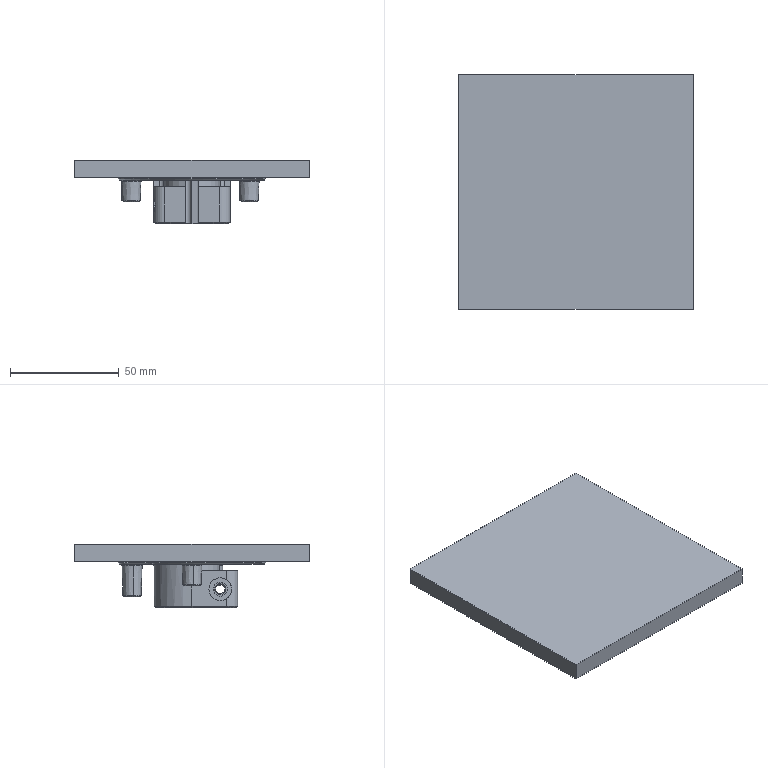NC program | NX | posted with a generic post | part box 108 x 108 x 29 mm
Lines 1 to 1353 of 23883:
N10 G17 G21 G94 G90
(FLOOR_WALL_COPY_COPY , TOOL : D63)
N12 T03 M6
N14 G54
N16 G17 G0 G90 X-68.5 Y33.999 S6500 M3
N18 G43 Z30. H3
N20 Z7.03
N22 G94 G1 Z4.03 F1250.
N24 X-65.5
N26 X65.5
N28 Y-8.8
N30 X-65.5
N32 X-68.5
N34 Z7.03
N36 G0 Z30.
N38 Y33.999
N40 Z6.06
N42 G1 Z3.06
N44 X-65.5
N46 X65.5
N48 Y-8.8
N50 X-65.5
N52 X-68.5
N54 Z6.06
N56 G0 Z30.
N58 Y33.999
N60 Z5.09
N62 G1 Z2.09
N64 X-65.5
N66 X65.5
N68 Y-8.8
N70 X-65.5
N72 X-68.5
N74 Z5.09
N76 G0 Z30.
N78 Y33.999
N80 Z4.12
N82 G1 Z1.12
N84 X-65.5
N86 X65.5
N88 Y-8.8
N90 X-65.5
N92 X-68.5
N94 Z4.12
N96 G0 Z30.
N98 Y33.999
N100 Z3.15
N102 G1 Z0.15
N104 X-65.5
N106 X65.5
N108 Y-8.8
N110 X-65.5
N112 X-68.5
N114 Z3.15
N116 G0 Z30.
(FLOOR_WALL_COPY_COPY_1 , TOOL : D63)
N118 X-68.499 Y33.998
N120 Z3.
N122 G1 Z0.
N124 X-65.499
N126 X65.499
N128 Y-8.799
N130 X-65.499
N132 X-68.499
N134 Z3.
N136 G0 Z30.
N138 M5
(CAVITY_MILL , TOOL : D10)
N140 T04 M6
N142 G54
N144 G17 G0 G90 X-40.997 Y12.31 S9500 M3
N146 G43 Z30. H4
N148 Z0.52
N150 G94 G1 Z-0.98 F1000.
N152 X-34.997 Y15.774
N154 G3 X-34.497 Y16.64 R1.
N156 G1 X-28.497
N158 Y2.421 F2500.
N160 X-28.709 Y-2.575
N162 G3 X-27.6 Y-2.498 R5.
N164 G1 Y-16.
N166 G3 X-26.755 Y-20.98 R15.1
N168 G2 X-29.497 Y-16.909 R34.
N170 G1 Y-2.478
N172 G3 X-28.709 Y-2.575 R5.
N174 G1 X-28.497 Y2.421
N176 G2 X-2.421 Y28.497 R28.6
N178 G1 X-16.64
N180 G3 X-28.497 Y16.64 R33.
N182 G1 X-34.497
N184 Y-18.192
N186 G3 X-18.192 Y-34.497 R39.
N188 G1 X18.192
N190 G3 X34.497 Y-18.192 R39.
N192 G1 Y2.421
N194 X28.497
N196 Y16.639
N198 G3 X25.153 Y16.744 R2.
N200 G1 X24.153 Y15.316
N202 G2 X28.497 Y2.421 R28.6
N204 G1 X28.709 Y-2.575
N206 G3 X29.497 Y-2.478 R5.
N208 G1 Y-16.909
N210 G2 X26.755 Y-20.98 R34.
N212 G3 X27.6 Y-16. R15.1
N214 G1 Y-2.498
N216 G3 X28.709 Y-2.575 R5.
N218 G1 X28.497 Y2.421
N220 X34.497
N222 Y18.192
N224 G3 X33.705 Y19.621 R39.
N226 X20.238 Y20.185 R8.
N228 G1 X16.737 Y15.186
N230 G2 X22.6 Y0. R22.6
N232 G1 Y-16.
N234 G2 X12.5 Y-26.1 R10.1
N236 G1 X3.
N238 G2 X0. Y-25.124 R5.1
N240 G1 X-0.067 Y-25.172
N242 G2 X-3. Y-26.1 R5.1
N244 G1 X-12.5
N246 G2 X-22.6 Y-16. R10.1
N248 G1 Y0.
N250 G2 X1.913 Y22.519 R22.6
N252 G1 X2.421 Y28.497
N254 G2 X6.132 Y27.935 R28.6
N256 G1 X6.526 Y28.497
N258 X2.421
N260 X1.913 Y22.519
N262 G2 X4.881 Y22.067 R22.6
N264 X8.546 Y20.922 R22.601
N266 G1 X12.046 Y25.921
N268 G3 X12.428 Y34.497 R8.
N270 G1 X-18.192
N272 G3 X-34.497 Y18.192 R39.
N274 G1 Y16.64
N276 G2 X-34.997 Y15.774 R1.
N278 G1 X-40.997 Y12.31
N280 Z0.52
N282 G0 Z-0.46
N284 G1 Z-1.96 F1000.
N286 X-34.997 Y15.774
N288 G3 X-34.497 Y16.64 R1.
N290 G1 X-28.497
N292 Y2.42 F2500.
N294 X-27.6 Y-2.499
N296 Y-16.
N298 G3 X-26.755 Y-20.98 R15.1
N300 G2 X-29.497 Y-16.909 R34.
N302 G1 Y-2.479
N304 G3 X-27.6 Y-2.499 R5.
N306 G1 X-28.497 Y2.42
N308 G2 X-2.42 Y28.497 R28.6
N310 G1 X-16.64
N312 G3 X-28.497 Y16.64 R33.
N314 G1 X-34.497
N316 Y-18.191
N318 G3 X-18.191 Y-34.497 R39.
N320 G1 X18.191
N322 G3 X34.497 Y-18.191 R39.
N324 G1 Y2.42
N326 X28.497
N328 Y16.639
N330 G3 X25.153 Y16.744 R2.
N332 G1 X24.153 Y15.316
N334 G2 X28.497 Y2.42 R28.6
N336 G1 X28.709 Y-2.576
N338 G3 X29.497 Y-2.479 R5.
N340 G1 Y-16.909
N342 G2 X26.755 Y-20.98 R34.
N344 G3 X27.6 Y-16. R15.1
N346 G1 Y-2.499
N348 G3 X28.709 Y-2.576 R5.
N350 G1 X28.497 Y2.42
N352 X34.497
N354 Y18.191
N356 G3 X33.705 Y19.621 R39.
N358 X20.238 Y20.185 R8.
N360 G1 X16.737 Y15.186
N362 G2 X22.6 Y0. R22.6
N364 G1 Y-16.
N366 G2 X12.5 Y-26.1 R10.1
N368 G1 X3.
N370 G2 X0. Y-25.124 R5.1
N372 G1 X-0.067 Y-25.172
N374 G2 X-3. Y-26.1 R5.1
N376 G1 X-12.5
N378 G2 X-22.6 Y-16. R10.1
N380 G1 Y0.
N382 G2 X1.912 Y22.519 R22.6
N384 G1 X2.42 Y28.497
N386 G2 X6.132 Y27.935 R28.6
N388 G1 X6.526 Y28.497
N390 X2.42
N392 X1.912 Y22.519
N394 G2 X5.91 Y21.813 R22.6
N396 X8.546 Y20.922 R22.601
N398 G1 X12.046 Y25.921
N400 G3 X12.428 Y34.497 R8.
N402 G1 X-18.191
N404 G3 X-34.497 Y18.191 R39.
N406 G1 Y16.64
N408 G2 X-34.997 Y15.774 R1.
N410 G1 X-40.997 Y12.31
N412 Z-0.46
N414 G0 X-40.998 Z-1.44
N416 G1 Z-2.94 F1000.
N418 X-34.998 Y15.774
N420 G3 X-34.498 Y16.64 R1.
N422 G1 X-28.498
N424 Y2.418 F2500.
N426 X-28.709 Y-2.577
N428 G3 X-27.6 Y-2.5 R5.
N430 G1 Y-16.
N432 G3 X-26.755 Y-20.98 R15.1
N434 G2 X-29.498 Y-16.908 R34.
N436 G1 Y-2.481
N438 G3 X-28.709 Y-2.577 R5.
N440 G1 X-28.498 Y2.418
N442 G2 X-2.418 Y28.498 R28.6
N444 G1 X-16.64
N446 G3 X-28.498 Y16.64 R33.
N448 G1 X-33.679 Y19.665
N450 G3 X-34.498 Y18.191 R39.
N452 G1 Y-18.191
N454 G3 X-18.191 Y-34.498 R39.
N456 G1 X18.191
N458 G3 X34.498 Y-18.191 R39.
N460 G1 Y2.418
N462 X28.498
N464 Y16.639
N466 G3 X25.153 Y16.744 R2.
N468 G1 X24.153 Y15.316
N470 G2 X28.498 Y2.418 R28.6
N472 G1 X28.709 Y-2.577
N474 G3 X29.498 Y-2.481 R5.
N476 G1 Y-16.908
N478 G2 X26.755 Y-20.98 R34.
N480 G3 X27.6 Y-16. R15.1
N482 G1 Y-2.5
N484 G3 X28.709 Y-2.577 R5.
N486 G1 X28.498 Y2.418
N488 X34.498
N490 Y18.191
N492 G3 X33.705 Y19.621 R39.
N494 X20.238 Y20.185 R8.
N496 G1 X16.737 Y15.186
N498 G2 X22.6 Y0. R22.6
N500 G1 Y-16.
N502 G2 X12.5 Y-26.1 R10.1
N504 G1 X3.
N506 G2 X0. Y-25.124 R5.1
N508 G1 X-0.067 Y-25.172
N510 G2 X-3. Y-26.1 R5.1
N512 G1 X-12.5
N514 G2 X-22.6 Y-16. R10.1
N516 G1 Y0.
N518 G2 X1.911 Y22.519 R22.6
N520 G1 X2.418 Y28.498
N522 G2 X6.132 Y27.935 R28.6
N524 G1 X6.526 Y28.498
N526 X2.418
N528 X1.911 Y22.519
N530 G2 X4.881 Y22.067 R22.6
N532 X8.546 Y20.922 R22.601
N534 G1 X12.046 Y25.921
N536 G3 X12.428 Y34.498 R8.
N538 G1 X-18.191
N540 G3 X-33.679 Y19.665 R39.
N542 G2 X-34.547 Y19.17 R1.
N544 G1 X-40.615 Y19.199
N546 Z-1.44
N548 G0 X-40.998 Y12.31 Z-2.42
N550 G1 Z-3.92 F1000.
N552 X-34.998 Y15.774
N554 G3 X-34.498 Y16.64 R1.
N556 G1 X-28.498
N558 Y2.417 F2500.
N560 X-28.709 Y-2.578
N562 G3 X-27.6 Y-2.502 R5.
N564 G1 Y-16.
N566 G3 X-26.755 Y-20.98 R15.1
N568 G2 X-29.498 Y-16.908 R34.
N570 G1 Y-2.482
N572 G3 X-28.709 Y-2.578 R5.
N574 G1 X-28.498 Y2.417
N576 G2 X-2.417 Y28.498 R28.6
N578 G1 X-16.64
N580 G3 X-28.498 Y16.64 R33.
N582 G1 X-33.679 Y19.665
N584 G3 X-34.498 Y18.191 R39.
N586 G1 Y-18.191
N588 G3 X-18.191 Y-34.498 R39.
N590 G1 X18.191
N592 G3 X34.498 Y-18.191 R39.
N594 G1 Y2.417
N596 X28.498
N598 Y16.639
N600 G3 X25.153 Y16.744 R2.
N602 G1 X24.153 Y15.316
N604 G2 X28.498 Y2.417 R28.6
N606 G1 X28.709 Y-2.578
N608 G3 X29.498 Y-2.482 R5.
N610 G1 Y-16.908
N612 G2 X26.755 Y-20.98 R34.
N614 G3 X27.6 Y-16. R15.1
N616 G1 Y-2.502
N618 G3 X28.709 Y-2.578 R5.
N620 G1 X28.498 Y2.417
N622 X34.498
N624 Y18.191
N626 G3 X33.705 Y19.621 R39.
N628 X20.238 Y20.185 R8.
N630 G1 X16.737 Y15.186
N632 G2 X22.6 Y0. R22.6
N634 G1 Y-16.
N636 G2 X12.5 Y-26.1 R10.1
N638 G1 X3.
N640 G2 X0. Y-25.124 R5.1
N642 G1 X-0.067 Y-25.172
N644 G2 X-3. Y-26.1 R5.1
N646 G1 X-12.5
N648 G2 X-22.6 Y-16. R10.1
N650 G1 Y0.
N652 G2 X1.91 Y22.519 R22.6
N654 G1 X2.417 Y28.498
N656 G2 X6.132 Y27.935 R28.6
N658 G1 X6.526 Y28.498
N660 X2.417
N662 X1.91 Y22.519
N664 G2 X4.881 Y22.067 R22.6
N666 X8.546 Y20.922 R22.601
N668 G1 X12.046 Y25.921
N670 G3 X12.428 Y34.498 R8.
N672 G1 X-18.191
N674 G3 X-33.679 Y19.665 R39.
N676 G2 X-34.548 Y19.169 R1.
N678 G1 X-40.615 Y19.199
N680 Z-2.42
N682 G0 X-40.998 Y12.309 Z-3.4
N684 G1 Z-4.9 F1000.
N686 X-34.998 Y15.774
N688 G3 X-34.498 Y16.64 R1.
N690 G1 X-28.498
N692 Y2.416 F2500.
N694 X-28.709 Y-2.58
N696 G3 X-27.6 Y-2.503 R5.
N698 G1 Y-16.
N700 G3 X-26.755 Y-20.98 R15.1
N702 G2 X-29.498 Y-16.908 R34.
N704 G1 Y-2.483
N706 G3 X-28.709 Y-2.58 R5.
N708 G1 X-28.498 Y2.416
N710 G2 X-2.416 Y28.498 R28.6
N712 G1 X-16.64
N714 G3 X-28.498 Y16.64 R33.
N716 G1 X-34.498
N718 Y-18.191
N720 G3 X-18.191 Y-34.498 R39.
N722 G1 X18.191
N724 G3 X34.498 Y-18.191 R39.
N726 G1 Y2.416
N728 X28.498
N730 Y16.639
N732 G3 X25.153 Y16.744 R2.
N734 G1 X24.153 Y15.316
N736 G2 X28.498 Y2.416 R28.6
N738 G1 X28.709 Y-2.58
N740 G3 X29.498 Y-2.483 R5.
N742 G1 Y-16.908
N744 G2 X26.755 Y-20.98 R34.
N746 G3 X27.6 Y-16. R15.1
N748 G1 Y-2.503
N750 G3 X28.709 Y-2.58 R5.
N752 G1 X28.498 Y2.416
N754 X34.498
N756 Y18.191
N758 G3 X33.705 Y19.621 R39.
N760 X20.238 Y20.185 R8.
N762 G1 X16.737 Y15.186
N764 G2 X22.6 Y0. R22.6
N766 G1 Y-16.
N768 G2 X12.5 Y-26.1 R10.1
N770 G1 X3.
N772 G2 X0. Y-25.124 R5.1
N774 G1 X-0.067 Y-25.172
N776 G2 X-3. Y-26.1 R5.1
N778 G1 X-12.5
N780 G2 X-22.6 Y-16. R10.1
N782 G1 Y0.
N784 G2 X1.909 Y22.519 R22.6
N786 G1 X2.416 Y28.498
N788 G2 X6.132 Y27.935 R28.6
N790 G1 X6.526 Y28.498
N792 X2.416
N794 X1.909 Y22.519
N796 G2 X4.881 Y22.067 R22.6
N798 X8.546 Y20.922 R22.601
N800 G1 X12.046 Y25.921
N802 G3 X12.428 Y34.498 R8.
N804 G1 X-18.191
N806 G3 X-34.498 Y18.191 R39.
N808 G1 Y16.64
N810 G2 X-34.998 Y15.774 R1.
N812 G1 X-40.998 Y12.309
N814 Z-3.4
N816 G0 Z-4.4
N818 G1 Z-5.9 F1000.
N820 X-34.998 Y15.773
N822 G3 X-34.498 Y16.639 R1.
N824 G1 X-28.498
N826 Y2.414 F2500.
N828 X-27.6 Y-2.504
N830 Y-16.
N832 G3 X-26.755 Y-20.98 R15.1
N834 G2 X-29.498 Y-16.908 R34.
N836 G1 Y-2.484
N838 G3 X-27.6 Y-2.504 R5.
N840 G1 X-28.498 Y2.414
N842 G2 X-18.95 Y21.421 R28.6
N844 X-20.167 Y26.121 R15.374
N846 G3 X-28.498 Y16.639 R33.
N848 G1 X-34.498
N850 Y-18.191
N852 G3 X-18.191 Y-34.498 R39.
N854 G1 X18.191
N856 G3 X34.498 Y-18.191 R39.
N858 G1 Y2.414
N860 X28.498
N862 Y16.639
N864 G3 X25.153 Y16.744 R2.
N866 G1 X24.153 Y15.316
N868 G2 X28.498 Y2.414 R28.6
N870 G1 X28.709 Y-2.581
N872 G3 X29.498 Y-2.484 R5.
N874 G1 Y-16.908
N876 G2 X26.755 Y-20.98 R34.
N878 G3 X27.6 Y-16. R15.1
N880 G1 Y-2.504
N882 G3 X28.709 Y-2.581 R5.
N884 G1 X28.498 Y2.414
N886 X34.498
N888 Y18.191
N890 G3 X33.705 Y19.621 R39.
N892 X20.238 Y20.185 R8.
N894 G1 X16.737 Y15.186
N896 G2 X22.6 Y0. R22.6
N898 G1 Y-16.
N900 G2 X12.5 Y-26.1 R10.1
N902 G1 X3.
N904 G2 X0. Y-25.124 R5.1
N906 G1 X-0.067 Y-25.172
N908 G2 X-3. Y-26.1 R5.1
N910 G1 X-12.5
N912 G2 X-22.6 Y-16. R10.1
N914 G1 Y0.
N916 G2 X-10.442 Y20.043 R22.6
N918 X2.957 Y22.406 R-9.374
N920 X4.243 Y22.198 R22.6
N922 X8.546 Y20.922 R22.601
N924 G1 X12.046 Y25.921
N926 G3 X12.428 Y34.498 R8.
N928 G1 X3.13
N930 G3 X-12.854 Y34.498 R10.574
N932 G1 X-18.191
N934 G3 X-34.498 Y18.191 R39.
N936 G1 Y16.639
N938 G2 X-34.998 Y15.773 R1.
N940 G1 X-40.998 Y12.309
N942 Z-4.4
N944 G0 Z-5.4
N946 G1 Z-6.9 F1000.
N948 X-34.998 Y15.773
N950 G3 X-34.498 Y16.639 R1.
N952 G1 X-28.498
N954 Y2.413 F2500.
N956 X-28.709 Y-2.582
N958 G3 X-27.6 Y-2.506 R5.
N960 G1 Y-16.
N962 G3 X-26.755 Y-20.98 R15.1
N964 G2 X-29.498 Y-16.908 R34.
N966 G1 Y-2.486
N968 G3 X-28.709 Y-2.582 R5.
N970 G1 X-28.498 Y2.413
N972 G2 X-18.971 Y21.402 R28.6
N974 X-20.191 Y26.102 R15.4
N976 G3 X-28.498 Y16.639 R33.
N978 G1 X-34.498
N980 Y-18.19
N982 G3 X-18.19 Y-34.498 R39.
N984 G1 X18.19
N986 G3 X34.498 Y-18.19 R39.
N988 G1 Y2.413
N990 X28.498
N992 Y16.638
N994 G3 X25.153 Y16.744 R2.
N996 G1 X24.153 Y15.316
N998 G2 X28.498 Y2.413 R28.6
N1000 G1 X28.709 Y-2.582
N1002 G3 X29.498 Y-2.486 R5.
N1004 G1 Y-16.908
N1006 G2 X26.755 Y-20.98 R34.
N1008 G3 X27.6 Y-16. R15.1
N1010 G1 Y-2.506
N1012 G3 X28.709 Y-2.582 R5.
N1014 G1 X28.498 Y2.413
N1016 X34.498
N1018 Y18.19
N1020 G3 X33.705 Y19.621 R39.
N1022 X20.238 Y20.185 R8.
N1024 G1 X16.737 Y15.186
N1026 G2 X22.6 Y0. R22.6
N1028 G1 Y-16.
N1030 G2 X12.5 Y-26.1 R10.1
N1032 G1 X3.
N1034 G2 X0. Y-25.124 R5.1
N1036 G1 X-0.067 Y-25.172
N1038 G2 X-3. Y-26.1 R5.1
N1040 G1 X-12.501
N1042 G2 X-22.6 Y-16. R10.1
N1044 G1 Y0.
N1046 G2 X-10.468 Y20.029 R22.6
N1048 X2.986 Y22.402 R-9.4
N1050 X4.27 Y22.193 R22.6
N1052 X8.546 Y20.922 R22.601
N1054 G1 X12.046 Y25.921
N1056 G3 X12.428 Y34.498 R8.
N1058 G1 X3.164
N1060 G3 X-12.888 Y34.498 R10.6
N1062 G1 X-18.19
N1064 G3 X-34.498 Y18.19 R39.
N1066 G1 Y16.639
N1068 G2 X-34.998 Y15.773 R1.
N1070 G1 X-40.998 Y12.309
N1072 Z-5.4
N1074 G0 Z-6.4
N1076 G1 Z-7.9 F1000.
N1078 X-34.998 Y15.773
N1080 G3 X-34.498 Y16.639 R1.
N1082 G1 X-28.498
N1084 Y2.412 F2500.
N1086 X-28.709 Y-2.584
N1088 G3 X-27.6 Y-2.507 R5.
N1090 G1 Y-16.
N1092 G3 X-26.755 Y-20.98 R15.1
N1094 G2 X-29.498 Y-16.907 R34.
N1096 G1 Y-2.487
N1098 G3 X-28.709 Y-2.584 R5.
N1100 G1 X-28.498 Y2.412
N1102 G2 X-18.992 Y21.384 R28.6
N1104 X-20.216 Y26.083 R15.426
N1106 G3 X-28.498 Y16.639 R33.
N1108 G1 X-34.498
N1110 Y-18.19
N1112 G3 X-18.19 Y-34.498 R39.
N1114 G1 X18.19
N1116 G3 X34.498 Y-18.19 R39.
N1118 G1 Y2.412
N1120 X28.498
N1122 Y16.638
N1124 G3 X25.153 Y16.744 R2.
N1126 G1 X24.153 Y15.316
N1128 G2 X28.498 Y2.412 R28.6
N1130 G1 X28.709 Y-2.584
N1132 G3 X29.498 Y-2.487 R5.
N1134 G1 Y-16.907
N1136 G2 X26.755 Y-20.98 R34.
N1138 G3 X27.6 Y-16. R15.1
N1140 G1 Y-2.507
N1142 G3 X28.709 Y-2.584 R5.
N1144 G1 X28.498 Y2.412
N1146 X34.498
N1148 Y18.19
N1150 G3 X33.705 Y19.621 R39.
N1152 X20.238 Y20.185 R8.
N1154 G1 X16.737 Y15.186
N1156 G2 X22.6 Y0. R22.6
N1158 G1 Y-16.
N1160 G2 X12.5 Y-26.1 R10.1
N1162 G1 X3.
N1164 G2 X0. Y-25.124 R5.1
N1166 G1 X-0.067 Y-25.172
N1168 G2 X-3. Y-26.1 R5.1
N1170 G1 X-12.5
N1172 G2 X-22.6 Y-16. R10.1
N1174 G1 Y0.
N1176 G2 X-10.494 Y20.016 R22.6
N1178 X3.015 Y22.398 R-9.426
N1180 X4.297 Y22.188 R22.6
N1182 X8.546 Y20.922 R22.601
N1184 G1 X12.046 Y25.921
N1186 G3 X12.428 Y34.498 R8.
N1188 G1 X3.199
N1190 G3 X-12.923 Y34.498 R10.626
N1192 G1 X-18.19
N1194 G3 X-34.498 Y18.19 R39.
N1196 G1 Y16.639
N1198 G2 X-34.998 Y15.773 R1.
N1200 G1 X-40.998 Y12.309
N1202 Z-6.4
N1204 G0 Z-7.4
N1206 G1 Z-8.9 F1000.
N1208 X-34.998 Y15.773
N1210 G3 X-34.498 Y16.639 R1.
N1212 G1 X-28.498
N1214 Y2.411 F2500.
N1216 X-27.6 Y-2.508
N1218 Y-16.
N1220 G3 X-26.755 Y-20.98 R15.1
N1222 G2 X-29.498 Y-16.907 R34.
N1224 G1 Y-2.488
N1226 G3 X-27.6 Y-2.508 R5.
N1228 G1 X-28.498 Y2.411
N1230 G2 X-19.012 Y21.366 R28.6
N1232 X-20.24 Y26.064 R15.452
N1234 G3 X-28.498 Y16.639 R33.
N1236 G1 X-34.498
N1238 Y-18.19
N1240 G3 X-18.19 Y-34.498 R39.
N1242 G1 X18.19
N1244 G3 X34.498 Y-18.19 R39.
N1246 G1 Y2.411
N1248 X28.498
N1250 Y16.638
N1252 G3 X25.153 Y16.744 R2.
N1254 G1 X24.153 Y15.316
N1256 G2 X28.498 Y2.411 R28.6
N1258 G1 X28.709 Y-2.585
N1260 G3 X29.498 Y-2.488 R5.
N1262 G1 Y-16.907
N1264 G2 X26.755 Y-20.98 R34.
N1266 G3 X27.6 Y-16. R15.1
N1268 G1 Y-2.508
N1270 G3 X28.709 Y-2.585 R5.
N1272 G1 X28.498 Y2.411
N1274 X34.498
N1276 Y18.19
N1278 G3 X33.705 Y19.621 R39.
N1280 X20.238 Y20.185 R8.
N1282 G1 X16.737 Y15.186
N1284 G2 X22.6 Y0. R22.6
N1286 G1 Y-16.
N1288 G2 X12.5 Y-26.1 R10.1
N1290 G1 X3.
N1292 G2 X0. Y-25.124 R5.1
N1294 G1 X-0.067 Y-25.172
N1296 G2 X-3. Y-26.1 R5.1
N1298 G1 X-12.5
N1300 G2 X-22.6 Y-16. R10.1
N1302 G1 Y0.
N1304 G2 X-10.52 Y20.002 R22.6
N1306 X3.044 Y22.394 R-9.452
N1308 X4.324 Y22.182 R22.6
N1310 X8.546 Y20.922 R22.601
N1312 G1 X12.046 Y25.921
N1314 G3 X12.428 Y34.498 R8.
N1316 G1 X3.233
N1318 G3 X-12.957 Y34.498 R10.652
N1320 G1 X-18.19
N1322 G3 X-34.498 Y18.19 R39.
N1324 G1 Y16.639
N1326 G2 X-34.998 Y15.773 R1.
N1328 G1 X-40.998 Y12.309
N1330 Z-7.4
N1332 G0 Z-8.4
N1334 G1 Z-9.9 F1000.
N1336 X-34.998 Y15.773
N1338 G3 X-34.498 Y16.639 R1.
N1340 G1 X-28.498
N1342 Y2.409 F2500.
N1344 X-27.6 Y-2.509
N1346 Y-16.
N1348 G3 X-26.755 Y-20.98 R15.1
N1350 G2 X-29.498 Y-16.907 R34.
N1352 G1 Y-2.49
N1354 G3 X-27.6 Y-2.509 R5.
N1356 G1 X-28.498 Y2.409
N1358 G2 X-19.032 Y21.348 R28.6
N1360 X-20.265 Y26.045 R15.478
N1362 G3 X-28.498 Y16.639 R33.
N1364 G1 X-34.498
N1366 Y-18.19
N1368 G3 X-18.19 Y-34.498 R39.
N1370 G1 X18.19
N1372 G3 X34.498 Y-18.19 R39.
N1374 G1 Y2.409
N1376 X28.498
N1378 Y16.638
N1380 G3 X25.153 Y16.744 R2.
N1382 G1 X24.153 Y15.316
N1384 G2 X28.498 Y2.409 R28.6
N1386 G1 X28.709 Y-2.586
N1388 G3 X29.498 Y-2.49 R5.
N1390 G1 Y-16.907
N1392 G2 X26.755 Y-20.98 R34.
N1394 G3 X27.6 Y-16. R15.1
N1396 G1 Y-2.509
N1398 G3 X28.709 Y-2.586 R5.
N1400 G1 X28.498 Y2.409
N1402 X34.498
N1404 Y18.19
N1406 G3 X33.705 Y19.621 R39.
N1408 X20.238 Y20.185 R8.
N1410 G1 X16.737 Y15.186
N1412 G2 X22.6 Y0. R22.6
N1414 G1 Y-16.
N1416 G2 X12.5 Y-26.1 R10.1
N1418 G1 X3.
N1420 G2 X0. Y-25.124 R5.1
N1422 G1 X-0.067 Y-25.172
N1424 G2 X-3. Y-26.1 R5.1
N1426 G1 X-12.5
N1428 G2 X-22.6 Y-16. R10.1
N1430 G1 Y0.
N1432 G2 X-10.545 Y19.989 R22.6
N1434 X3.072 Y22.39 R-9.478
N1436 X4.351 Y22.177 R22.6
N1438 X8.546 Y20.922 R22.601
N1440 G1 X12.046 Y25.921
N1442 G3 X12.428 Y34.498 R8.
N1444 G1 X3.267
N1446 G3 X-12.991 Y34.498 R10.678
N1448 G1 X-18.19
N1450 G3 X-34.498 Y18.19 R39.
N1452 G1 Y16.639
N1454 G2 X-34.998 Y15.773 R1.
N1456 G1 X-40.998 Y12.309
N1458 Z-8.4
N1460 G0 Y12.308 Z-9.4
N1462 G1 Z-10.9 F1000.
N1464 X-34.998 Y15.772
N1466 G3 X-34.498 Y16.638 R1.
N1468 G1 X-28.498
N1470 Y5.649 F2500.
N1472 G2 X-28.024 Y5.709 R15.381
N1474 X-19.053 Y21.329 R28.6
N1476 X-20.289 Y26.026 R15.505
N1478 G3 X-28.498 Y16.638 R33.
N1480 G1 X-33.68 Y19.664
N1482 G3 X-34.498 Y18.189 R39.
N1484 G1 Y-2.873
N1486 G3 X-34.498 Y-16.28 R10.581
N1488 G1 Y-18.189
N1490 G3 X-18.189 Y-34.498 R39.
N1492 G1 X18.189
N1494 G3 X34.498 Y-18.189 R39.
N1496 G1 Y-8.351
N1498 G3 X34.498 Y8.351 R10.581
N1500 G1 Y15.373
N1502 X28.498
N1504 Y16.638
N1506 G3 X25.153 Y16.744 R2.
N1508 G1 X24.153 Y15.316
N1510 G2 X24.382 Y14.95 R28.6
N1512 X28.498 Y15.373 R15.381
N1514 G1 X34.498
N1516 Y18.189
N1518 G3 X33.705 Y19.621 R39.
N1520 X20.238 Y20.185 R8.
N1522 G1 X16.737 Y15.186
N1524 G2 X21.549 Y6.812 R22.6
N1526 X22.605 Y-7.675 R-9.381
N1528 G1 X22.6 Y-7.682
N1530 Y-16.
N1532 G2 X22.035 Y-19.331 R10.1
N1534 G1 X28.324 Y-16.786
N1536 X22.035 Y-19.331
N1538 G2 X12.5 Y-26.1 R10.1
N1540 G1 X3.
N1542 G2 X0. Y-25.124 R5.1
N1544 G1 X-0.067 Y-25.172
N1546 G2 X-3. Y-26.1 R5.1
N1548 G1 X-12.5
N1550 G2 X-22.38 Y-18.095 R10.1
N1552 X-22.6 Y-0.96 R-9.381
N1554 G1 Y0.
N1556 G2 X-10.571 Y19.975 R22.6
N1558 X3.101 Y22.386 R-9.505
N1560 X7.143 Y21.442 R22.6
N1562 X8.546 Y20.922 R22.601
N1564 G1 X12.046 Y25.921
N1566 G3 X12.427 Y34.498 R8.
N1568 G1 X3.302
N1570 G3 X-13.026 Y34.498 R10.705
N1572 G1 X-18.189
N1574 G3 X-33.68 Y19.664 R39.
N1576 G2 X-34.548 Y19.168 R1.
N1578 G1 X-40.615 Y19.197
N1580 Z-9.4
N1582 G0 X-40.999 Y12.308 Z-10.4
N1584 G1 Z-11.9 F1000.
N1586 X-34.999 Y15.772
N1588 G3 X-34.499 Y16.638 R1.
N1590 G1 X-28.499
N1592 Y5.684 F2500.
N1594 G2 X-28.017 Y5.745 R15.416
N1596 X-19.074 Y21.311 R28.6
N1598 X-20.314 Y26.007 R15.531
N1600 G3 X-28.499 Y16.638 R33.
N1602 G1 X-33.68 Y19.663
N1604 G3 X-34.499 Y18.189 R39.
N1606 G1 Y-2.818
N1608 G3 X-34.499 Y-16.335 R10.616
N1610 G1 Y-18.189
N1612 G3 X-18.189 Y-34.499 R39.
N1614 G1 X18.189
N1616 G3 X30.69 Y-24.065 R39.
N1618 G1 X28.322 Y-16.804
N1620 X30.69 Y-24.065
N1622 G3 X34.499 Y-18.189 R39.
N1624 G1 Y-8.395
N1626 G3 X34.499 Y8.395 R10.616
N1628 G1 Y15.408
N1630 X28.499
N1632 Y16.638
N1634 G3 X25.153 Y16.744 R2.
N1636 G1 X24.153 Y15.316
N1638 G2 X24.362 Y14.981 R28.6
N1640 X28.499 Y15.408 R15.416
N1642 G1 X34.499
N1644 Y18.189
N1646 G3 X33.705 Y19.621 R39.
N1648 X20.238 Y20.185 R8.
N1650 G1 X16.737 Y15.186
N1652 G2 X21.537 Y6.849 R22.6
N1654 X22.6 Y-7.714 R-9.416
N1656 G1 Y-8.798
N1658 Y-16.
N1660 G2 X12.5 Y-26.1 R10.1
N1662 G1 X2.915 Y-26.099
N1664 G2 X0. Y-25.124 R5.1
N1666 G1 X-0.067 Y-25.172
N1668 G2 X-3. Y-26.1 R5.1
N1670 G1 X-12.5
N1672 G2 X-22.373 Y-18.13 R10.1
N1674 X-22.6 Y-0.922 R-9.416
N1676 G1 Y0.
N1678 G2 X-10.596 Y19.962 R22.6
N1680 X3.13 Y22.382 R-9.531
N1682 X5.576 Y21.901 R22.6
N1684 X8.546 Y20.922 R22.601
N1686 G1 X12.046 Y25.921
N1688 G3 X12.427 Y34.499 R8.
N1690 G1 X3.336
N1692 G3 X-13.06 Y34.499 R10.731
N1694 G1 X-18.189
N1696 G3 X-33.68 Y19.663 R39.
N1698 G2 X-34.549 Y19.168 R1.
N1700 G1 X-40.615 Y19.197
N1702 Z-10.4
N1704 G0 X-40.999 Y12.308 Z-11.4
N1706 G1 Z-12.9 F1000.
N1708 X-34.999 Y15.772
N1710 G3 X-34.499 Y16.638 R1.
N1712 G1 X-28.499
N1714 Y5.719 F2500.
N1716 G2 X-28.01 Y5.781 R15.451
N1718 X-19.094 Y21.292 R28.6
N1720 X-20.338 Y25.988 R15.557
N1722 G3 X-28.499 Y16.638 R33.
N1724 G1 X-33.68 Y19.663
N1726 G3 X-34.499 Y18.189 R39.
N1728 G1 Y-2.763
N1730 G3 X-34.499 Y-16.39 R10.651
N1732 G1 Y-18.189
N1734 G3 X-18.189 Y-34.499 R39.
N1736 G1 X18.189
N1738 G3 X34.499 Y-18.189 R39.
N1740 G1 Y-8.439
N1742 G3 X34.499 Y8.439 R10.651
N1744 G1 Y15.443
N1746 X28.499
N1748 Y16.637
N1750 G3 X25.153 Y16.744 R2.
N1752 G1 X24.153 Y15.316
N1754 X24.343 Y15.012
N1756 G2 X28.499 Y15.443 R15.451
N1758 G1 X34.499
N1760 Y18.189
N1762 G3 X33.705 Y19.621 R39.
N1764 X20.238 Y20.185 R8.
N1766 G1 X16.737 Y15.186
N1768 G2 X21.526 Y6.885 R22.6
N1770 X22.6 Y-7.757 R-9.451
N1772 G1 Y-8.799
N1774 Y-16.
N1776 G2 X22.035 Y-19.331 R10.1
N1778 G1 X28.32 Y-16.823
N1780 X22.035 Y-19.331
N1782 G2 X12.5 Y-26.1 R10.1
N1784 G1 X3.
N1786 G2 X0. Y-25.124 R5.1
N1788 G1 X-0.067 Y-25.172
N1790 G2 X-3. Y-26.1 R5.1
N1792 G1 X-12.5
N1794 G2 X-22.365 Y-18.165 R10.1
N1796 X-22.6 Y-0.884 R-9.451
N1798 G1 Y0.
N1800 G2 X-10.622 Y19.948 R22.6
N1802 X3.159 Y22.378 R-9.557
N1804 X5.474 Y21.927 R22.6
N1806 X8.546 Y20.922 R22.601
N1808 G1 X12.046 Y25.921
N1810 G3 X12.427 Y34.499 R8.
N1812 G1 X3.37
N1814 G3 X-13.094 Y34.499 R10.757
N1816 G1 X-18.189
N1818 G3 X-33.68 Y19.663 R39.
N1820 G2 X-34.549 Y19.167 R1.
N1822 G1 X-40.615 Y19.197
N1824 Z-11.4
N1826 G0 X-40.999 Y12.308 Z-12.4
N1828 G1 Z-13.9 F1000.
N1830 X-34.999 Y15.772
N1832 G3 X-34.499 Y16.638 R1.
N1834 G1 X-28.499
N1836 Y5.754 F2500.
N1838 G2 X-28.002 Y5.817 R15.486
N1840 X-19.115 Y21.274 R28.6
N1842 X-20.362 Y25.969 R15.583
N1844 G3 X-28.499 Y16.638 R33.
N1846 G1 X-34.499
N1848 Y-2.709
N1850 G3 X-34.499 Y-16.444 R10.686
N1852 G1 Y-18.189
N1854 G3 X-18.189 Y-34.499 R39.
N1856 G1 X18.189
N1858 G3 X30.69 Y-24.065 R39.
N1860 G1 X28.318 Y-16.841
N1862 X30.69 Y-24.065
N1864 G3 X34.499 Y-18.189 R39.
N1866 G1 Y-8.483
N1868 G3 X34.499 Y8.483 R10.686
N1870 G1 Y15.478
N1872 X28.499
N1874 Y16.637
N1876 G3 X25.153 Y16.744 R2.
N1878 G1 X24.153 Y15.316
N1880 X24.324 Y15.044
N1882 G2 X28.499 Y15.478 R15.486
N1884 G1 X34.499
N1886 Y18.189
N1888 G3 X33.705 Y19.621 R39.
N1890 X20.238 Y20.185 R8.
N1892 G1 X16.737 Y15.186
N1894 G2 X21.514 Y6.922 R22.6
N1896 X22.6 Y-7.799 R-9.486
N1898 G1 Y-16.
N1900 G2 X12.5 Y-26.1 R10.1
N1902 G1 X3.
N1904 G2 X0. Y-25.124 R5.1
N1906 G1 X-0.067 Y-25.172
N1908 G2 X-3. Y-26.1 R5.1
N1910 G1 X-12.5
N1912 G2 X-22.358 Y-18.2 R10.1
N1914 X-22.6 Y-0.846 R-9.486
N1916 G1 Y0.
N1918 G2 X-10.647 Y19.935 R22.6
N1920 X3.187 Y22.374 R-9.583
N1922 X7.802 Y21.211 R22.6
N1924 X8.546 Y20.922 R22.601
N1926 G1 X12.046 Y25.921
N1928 G3 X12.427 Y34.499 R8.
N1930 G1 X3.404
N1932 G3 X-13.128 Y34.499 R10.783
N1934 G1 X-18.189
N1936 G3 X-34.499 Y18.189 R39.
N1938 G1 Y16.638
N1940 G2 X-34.999 Y15.772 R1.
N1942 G1 X-40.999 Y12.308
N1944 Z-12.4
N1946 G0 Z-13.4
N1948 G1 Z-14.9 F1000.
N1950 X-34.999 Y15.772
N1952 G3 X-34.499 Y16.638 R1.
N1954 G1 X-28.499
N1956 Y5.79 F2500.
N1958 G2 X-27.995 Y5.853 R15.521
N1960 X-19.135 Y21.256 R28.6
N1962 X-20.387 Y25.95 R15.609
N1964 G3 X-28.499 Y16.638 R33.
N1966 G1 X-33.681 Y19.663
N1968 G3 X-34.499 Y18.189 R39.
N1970 G1 Y-2.655
N1972 G3 X-36.872 Y-7.731 R10.721
N1974 X-34.499 Y-16.499 R10.721
N1976 G1 Y-18.189
N1978 G3 X-18.189 Y-34.499 R39.
N1980 G1 X18.189
N1982 G3 X34.499 Y-18.189 R39.
N1984 G1 Y-8.527
N1986 G3 X34.499 Y8.527 R10.721
N1988 G1 Y15.513
N1990 X28.499
N1992 Y16.637
N1994 G3 X25.153 Y16.744 R2.
N1996 G1 X24.153 Y15.316
N1998 X24.305 Y15.075
N2000 G2 X28.499 Y15.513 R15.521
N2002 G1 X34.499
N2004 Y18.189
N2006 G3 X33.705 Y19.621 R39.
N2008 X20.238 Y20.185 R8.
N2010 G1 X16.737 Y15.186
N2012 G2 X21.502 Y6.959 R22.6
N2014 X22.6 Y-7.842 R-9.521
N2016 G1 Y-8.799
N2018 Y-9.262
N2020 Y-16.
N2022 G2 X22.035 Y-19.331 R10.1
N2024 G1 X28.317 Y-16.86
N2026 X22.035 Y-19.331
N2028 G2 X12.5 Y-26.1 R10.1
N2030 G1 X3.
N2032 G2 X0. Y-25.124 R5.1
N2034 G1 X-0.067 Y-25.172
N2036 G2 X-3. Y-26.1 R5.1
N2038 G1 X-12.5
N2040 G2 X-22.35 Y-18.235 R10.1
N2042 X-35.69 Y-7.937 R9.521
N2044 X-22.6 Y-0.809 R9.521
N2046 G1 Y0.
N2048 G2 X-10.673 Y19.921 R22.6
N2050 X3.216 Y22.37 R-9.609
N2052 X8.546 Y20.922 R22.601
N2054 G1 X12.046 Y25.921
N2056 G3 X12.427 Y34.499 R8.
N2058 G1 X3.438
N2060 G3 X-13.162 Y34.499 R10.809
N2062 G1 X-18.189
N2064 G3 X-33.681 Y19.663 R39.
N2066 G2 X-34.549 Y19.167 R1.
N2068 G1 X-40.616 Y19.196
N2070 Z-13.4
N2072 G0 X-40.999 Y12.307 Z-14.4
N2074 G1 Z-15.9 F1000.
N2076 X-34.999 Y15.771
N2078 G3 X-34.499 Y16.638 R1.
N2080 G1 X-28.499
N2082 Y5.825 F2500.
N2084 G2 X-27.987 Y5.889 R15.556
N2086 X-19.156 Y21.237 R28.6
N2088 X-20.411 Y25.931 R15.635
N2090 G3 X-28.499 Y16.638 R33.
N2092 G1 X-34.499
N2094 Y-2.601
N2096 G3 X-34.499 Y-16.552 R10.756
N2098 G1 Y-18.188
N2100 G3 X-18.188 Y-34.499 R39.
N2102 G1 X18.188
N2104 G3 X34.499 Y-18.188 R39.
N2106 G1 Y-8.571
N2108 G3 X34.499 Y8.571 R10.756
N2110 G1 Y15.548
N2112 X28.499
N2114 Y16.637
N2116 G3 X25.153 Y16.744 R2.
N2118 G1 X24.153 Y15.316
N2120 X24.285 Y15.106
N2122 G2 X28.499 Y15.548 R15.556
N2124 G1 X34.499
N2126 Y18.188
N2128 G3 X33.705 Y19.621 R39.
N2130 X20.238 Y20.185 R8.
N2132 G1 X16.737 Y15.186
N2134 G2 X21.49 Y6.996 R22.6
N2136 X22.6 Y-7.884 R-9.556
N2138 G1 Y-8.799
N2140 Y-16.
N2142 G2 X22.035 Y-19.331 R10.1
N2144 G1 X28.315 Y-16.879
N2146 X22.035 Y-19.331
N2148 G2 X12.5 Y-26.1 R10.1
N2150 G1 X3.
N2152 G2 X0. Y-25.124 R5.1
N2154 G1 X-0.067 Y-25.172
N2156 G2 X-3. Y-26.1 R5.1
N2158 G1 X-12.5
N2160 G2 X-22.342 Y-18.269 R10.1
N2162 X-22.6 Y-0.771 R-9.556
N2164 G1 Y0.
N2166 G2 X-10.698 Y19.908 R22.6
N2168 X3.244 Y22.366 R-9.635
N2170 X4.514 Y22.145 R22.6
N2172 X8.546 Y20.922 R22.601
N2174 G1 X12.046 Y25.921
N2176 G3 X12.427 Y34.499 R8.
N2178 G1 X3.472
N2180 G3 X-13.196 Y34.499 R10.835
N2182 G1 X-18.188
N2184 G3 X-34.499 Y18.188 R39.
N2186 G1 Y16.638
N2188 G2 X-34.999 Y15.771 R1.
N2190 G1 X-40.999 Y12.307
N2192 Z-14.4
N2194 G0 Z-15.4
N2196 G1 Z-16.9 F1000.
N2198 X-34.999 Y15.771
N2200 G3 X-34.499 Y16.637 R1.
N2202 G1 X-28.499
N2204 Y5.86 F2500.
N2206 G2 X-27.98 Y5.925 R15.591
N2208 X-19.176 Y21.219 R28.6
N2210 X-20.435 Y25.912 R15.661
N2212 G3 X-28.499 Y16.637 R33.
N2214 G1 X-34.499
N2216 Y-2.548
N2218 G3 X-34.499 Y-16.605 R10.791
N2220 G1 Y-18.188
N2222 G3 X-18.188 Y-34.499 R39.
N2224 G1 X18.188
N2226 G3 X30.69 Y-24.065 R39.
N2228 G1 X28.313 Y-16.897
N2230 X30.69 Y-24.065
N2232 G3 X34.499 Y-18.188 R39.
N2234 G1 Y-8.614
N2236 G3 X34.499 Y8.614 R10.791
N2238 G1 Y15.583
N2240 X28.499
N2242 Y16.637
N2244 G3 X25.153 Y16.744 R2.
N2246 G1 X24.153 Y15.316
N2248 X24.266 Y15.137
N2250 G2 X28.499 Y15.583 R15.591
N2252 G1 X34.499
N2254 Y18.188
N2256 G3 X33.705 Y19.621 R39.
N2258 X20.238 Y20.185 R8.
N2260 G1 X16.737 Y15.186
N2262 G2 X21.478 Y7.032 R22.6
N2264 X22.6 Y-7.926 R-9.591
N2266 G1 Y-8.799
N2268 Y-16.
N2270 G2 X12.5 Y-26.1 R10.1
N2272 G1 X3.
N2274 G2 X0. Y-25.124 R5.1
N2276 G1 X-0.067 Y-25.172
N2278 G2 X-3. Y-26.1 R5.1
N2280 G1 X-12.5
N2282 G2 X-22.334 Y-18.304 R10.1
N2284 X-22.6 Y-0.733 R-9.591
N2286 G1 Y0.
N2288 G2 X-10.723 Y19.894 R22.6
N2290 X3.272 Y22.362 R-9.661
N2292 X4.541 Y22.139 R22.6
N2294 X8.546 Y20.922 R22.601
N2296 G1 X12.046 Y25.921
N2298 G3 X12.427 Y34.499 R8.
N2300 G1 X3.506
N2302 G3 X-13.23 Y34.499 R10.861
N2304 G1 X-18.188
N2306 G3 X-34.499 Y18.188 R39.
N2308 G1 Y16.637
N2310 G2 X-34.999 Y15.771 R1.
N2312 G1 X-40.999 Y12.307
N2314 Z-15.4
N2316 G0 Z-16.4
N2318 G1 Z-17.9 F1000.
N2320 X-34.999 Y15.771
N2322 G3 X-34.499 Y16.637 R1.
N2324 G1 X-28.499
N2326 Y5.895 F2500.
N2328 G2 X-27.972 Y5.961 R15.626
N2330 X-19.197 Y21.2 R28.6
N2332 X-20.46 Y25.892 R15.688
N2334 G3 X-28.499 Y16.637 R33.
N2336 G1 X-34.499
N2338 Y-2.494
N2340 G3 X-34.499 Y-16.659 R10.826
N2342 G1 Y-18.188
N2344 G3 X-18.188 Y-34.499 R39.
N2346 G1 X18.188
N2348 G3 X34.499 Y-18.188 R39.
N2350 G1 Y-8.658
N2352 G3 X34.499 Y8.658 R10.826
N2354 G1 Y15.618
N2356 X28.499
N2358 Y16.636
N2360 G3 X25.153 Y16.744 R2.
N2362 G1 X24.153 Y15.316
N2364 X24.246 Y15.168
N2366 G2 X28.499 Y15.618 R15.626
N2368 G1 X34.499
N2370 Y18.188
N2372 G3 X33.705 Y19.621 R39.
N2374 X20.238 Y20.185 R8.
N2376 G1 X16.737 Y15.186
N2378 G2 X21.466 Y7.069 R22.6
N2380 X22.6 Y-7.969 R-9.626
N2382 G1 Y-16.
N2384 G2 X22.035 Y-19.331 R10.1
N2386 G1 X28.311 Y-16.916
N2388 X22.035 Y-19.331
N2390 G2 X12.5 Y-26.1 R10.1
N2392 G1 X3.
N2394 G2 X0. Y-25.124 R5.1
N2396 G1 X-0.067 Y-25.172
N2398 G2 X-3. Y-26.1 R5.1
N2400 G1 X-12.5
N2402 G2 X-22.326 Y-18.339 R10.1
N2404 X-22.6 Y-0.695 R-9.626
N2406 G1 Y0.
N2408 G2 X-10.749 Y19.88 R22.6
N2410 X3.301 Y22.358 R-9.688
N2412 X4.569 Y22.133 R22.6
N2414 X8.546 Y20.922 R22.601
N2416 G1 X12.046 Y25.921
N2418 G3 X12.427 Y34.499 R8.
N2420 G1 X3.54
N2422 G3 X-13.264 Y34.499 R10.888
N2424 G1 X-18.188
N2426 G3 X-34.499 Y18.188 R39.
N2428 G1 Y16.637
N2430 G2 X-34.999 Y15.771 R1.
N2432 G1 X-40.999 Y12.307
N2434 Z-16.4
N2436 G0 Z-17.4
N2438 G1 Z-18.9 F1000.
N2440 X-34.999 Y15.771
N2442 G3 X-34.499 Y16.637 R1.
N2444 G1 X-28.499
N2446 Y5.931 F2500.
N2448 G2 X-27.964 Y5.997 R15.661
N2450 X-19.217 Y21.182 R28.6
N2452 X-20.484 Y25.873 R15.714
N2454 G3 X-28.499 Y16.637 R33.
N2456 G1 X-34.499
N2458 Y-2.441
N2460 G3 X-34.499 Y-16.712 R10.861
N2462 G1 Y-18.188
N2464 G3 X-18.188 Y-34.499 R39.
N2466 G1 X18.188
N2468 G3 X30.69 Y-24.065 R39.
N2470 G1 X28.309 Y-16.935
N2472 X30.69 Y-24.065
N2474 G3 X34.499 Y-18.188 R39.
N2476 G1 Y-8.702
N2478 G3 X34.499 Y8.702 R10.861
N2480 G1 Y15.653
N2482 X28.499
N2484 Y16.636
N2486 G3 X25.153 Y16.744 R2.
N2488 G1 X24.153 Y15.316
N2490 X24.227 Y15.2
N2492 G2 X28.499 Y15.653 R15.661
N2494 G1 X34.499
N2496 Y18.188
N2498 G3 X33.705 Y19.621 R39.
N2500 X20.238 Y20.185 R8.
N2502 G1 X16.737 Y15.186
N2504 G2 X21.454 Y7.105 R22.6
N2506 X22.6 Y-8.011 R-9.661
N2508 G1 Y-9.423
N2510 Y-16.
N2512 G2 X12.5 Y-26.1 R10.1
N2514 G1 X3.
N2516 G2 X0. Y-25.124 R5.1
N2518 G1 X-0.061 Y-25.168
N2520 G2 X-3. Y-26.1 R5.1
N2522 G1 X-12.5
N2524 G2 X-22.317 Y-18.373 R10.1
N2526 X-22.6 Y-0.657 R-9.661
N2528 G1 Y0.
N2530 G2 X-10.774 Y19.867 R22.6
N2532 X3.329 Y22.353 R-9.714
N2534 X8.546 Y20.922 R22.601
N2536 G1 X12.046 Y25.921
N2538 G3 X12.427 Y34.499 R8.
N2540 G1 X3.574
N2542 G3 X-13.298 Y34.499 R10.914
N2544 G1 X-18.188
N2546 G3 X-34.499 Y18.188 R39.
N2548 G1 Y16.637
N2550 G2 X-34.999 Y15.771 R1.
N2552 G1 X-40.999 Y12.307
N2554 Z-17.4
N2556 G0 Z-18.4
N2558 G1 Z-19.9 F1000.
N2560 X-34.999 Y15.771
N2562 G3 X-34.499 Y16.637 R1.
N2564 G1 X-28.499
N2566 Y6.5 F2500.
N2568 G2 X-27.834 Y6.577 R16.225
N2570 X-19.651 Y20.78 R28.6
N2572 X-20.999 Y25.457 R16.275
N2574 G3 X-28.499 Y16.637 R33.
N2576 G1 X-33.681 Y19.662
N2578 G3 X-34.499 Y18.188 R39.
N2580 G1 Y-1.609
N2582 G3 X-37.733 Y-9.861 R11.425
N2584 X-35.243 Y-16.701 R39.
N2586 X-34.499 Y-17.544 R11.425
N2588 G1 Y-18.188
N2590 G3 X-18.188 Y-34.499 R39.
N2592 G1 X18.188
N2594 G3 X34.499 Y-18.188 R39.
N2596 G1 Y-9.396
N2598 G3 X38.83 Y-3.64 R11.425
N2600 X38.999 Y-0.209 R39.
N2602 G1 Y0.209
N2604 G3 X38.83 Y3.64 R39.
N2606 X34.499 Y9.396 R11.425
N2608 G1 Y16.217
N2610 X28.499
N2612 Y16.636
N2614 G3 X25.153 Y16.744 R2.
N2616 G1 X24.526 Y15.849
N2618 G2 X28.499 Y16.217 R16.225
N2620 G1 X34.499
N2622 Y18.188
N2624 G3 X33.705 Y19.621 R39.
N2626 X20.238 Y20.185 R8.
N2628 G1 X16.737 Y15.186
N2630 G2 X21.254 Y7.684 R22.6
N2632 X22.6 Y-8.683 R-10.225
N2634 G1 Y-10.068
N2636 Y-16.
N2638 G2 X22.035 Y-19.331 R10.1
N2640 G1 X28.273 Y-17.241
N2642 X22.035 Y-19.331
N2644 G2 X12.5 Y-26.1 R10.1
N2646 G1 X3.
N2648 G2 X0. Y-25.124 R5.1
N2650 G1 X-0.061 Y-25.168
N2652 G2 X-3. Y-26.1 R5.1
N2654 G1 X-12.5
N2656 G2 X-22.167 Y-18.924 R10.1
N2658 X-22.6 Y-0.049 R-10.225
N2660 G1 Y0.
N2662 G2 X-11.304 Y19.57 R22.6
N2664 X3.929 Y22.256 R-10.275
N2666 X8.546 Y20.922 R22.601
N2668 G1 X12.046 Y25.921
N2670 G3 X12.427 Y34.499 R8.
N2672 G1 X4.288
N2674 G3 X-2.946 Y38.889 R11.475
N2676 X-10.532 Y37.551 R39.
N2678 X-14.012 Y34.499 R11.475
N2680 G1 X-18.188
N2682 G3 X-33.681 Y19.662 R39.
N2684 G2 X-34.55 Y19.166 R1.
N2686 G1 X-40.616 Y19.195
N2688 Z-18.4
N2690 G0 Z30.
N2692 M5